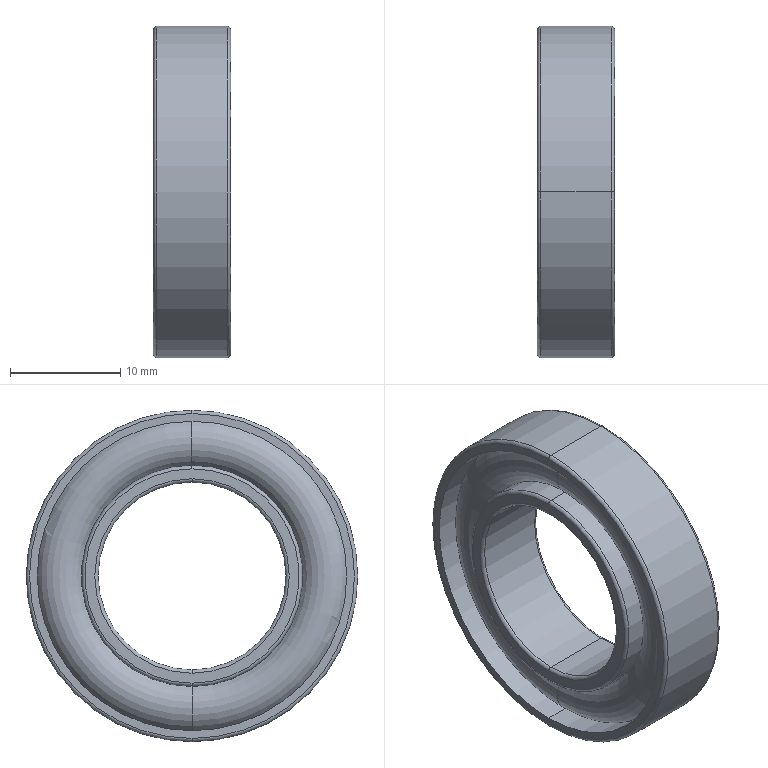Part | STEP file | QA-Bearing-B6903ZZ | 1 solid | 32 faces | box 7 x 30 x 30 mm | volume 2496 mm3 | torus 16 | cylinder 12 | plane 4 | commonest cylinder face diameters 20 x4 28 x4 17 x2 30 x2